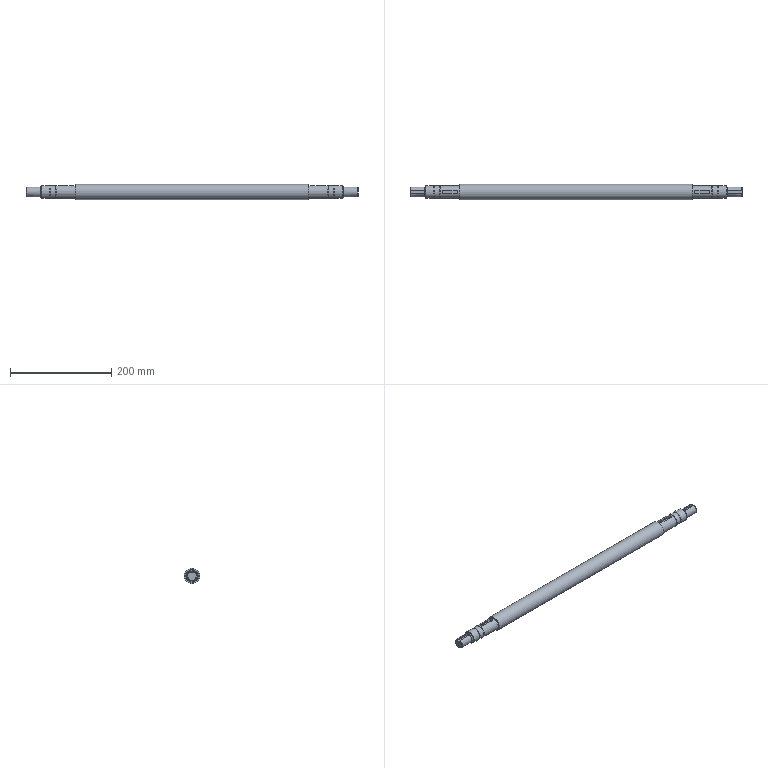CAM job | NX | 3-axis milling | part box 656 x 30.5 x 30.5 mm | stock box 758.463 x 30.5 x 30.5 mm
Tools:
number,name,description,diameter,corner_radius,flute_length,length,flutes
4,D4,Milling Tool-5 Parameters,4.0,0.0,50.0,75.0,2
5,D4JING,Milling Tool-5 Parameters,5.0,0.0,50.0,75.0,2
2,D6A45,Milling Tool-5 Parameters,6.0,0.0,3.0,3.0,2
Operations:
program,operation,operation_type,tool,method,geometry_group,spindle_rpm,surface_speed,feed_per_tooth,feed_cut,feed_plunge,cut_length_mm,path_length_mm,cut_time_min,machine_time_min
1,ZLEVEL_PROFILE,ZLevelMilling,D4,METHOD,A,4000.0,50.0,0.175,1400.0,1000.0,4774.914,5417.834,3.422,3.487
1,ZLEVEL_PROFILE_COPY,ZLevelMilling,D4,METHOD,A,4000.0,50.0,0.175,1400.0,1000.0,5394.416,6252.733,3.879,3.965
1,ZLEVEL_PROFILE_COPY_COPY,ZLevelMilling,D4JING,METHOD,A,5000.0,78.0,0.1,1000.0,1000.0,129.806,945.913,0.1298,0.2114
1,ZLEVEL_PROFILE_COPY_COPY_COPY,ZLevelMilling,D4JING,METHOD,A,5000.0,78.0,0.1,1000.0,1000.0,113.955,752.032,0.114,0.1778
1,ZLEVEL_PROFILE_1_COPY_1_COPY,ZLevelMilling,D6A45,METHOD,A,7500.0,141.0,0.0667,1000.0,100.0,133.517,762.853,0.1335,0.1965
1,ZLEVEL_PROFILE_1_COPY_1_COPY_COPY,ZLevelMilling,D6A45,METHOD,A,7500.0,141.0,0.0667,1000.0,100.0,127.629,1079.141,0.1276,0.2228